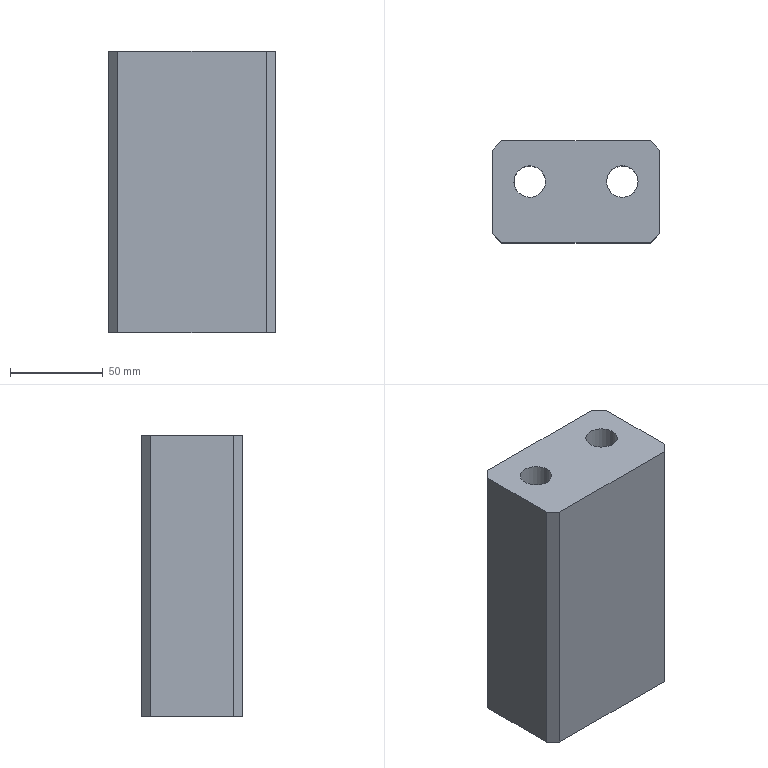Part | STEP file | 1_id1482_x_t | 1 solid | 22 faces | box 90 x 55 x 152 mm | volume 644176 mm3 | plane 12 | cylinder 7 | cone 3 | commonest cylinder face diameters 10.25 x3 17 x2 24 x2